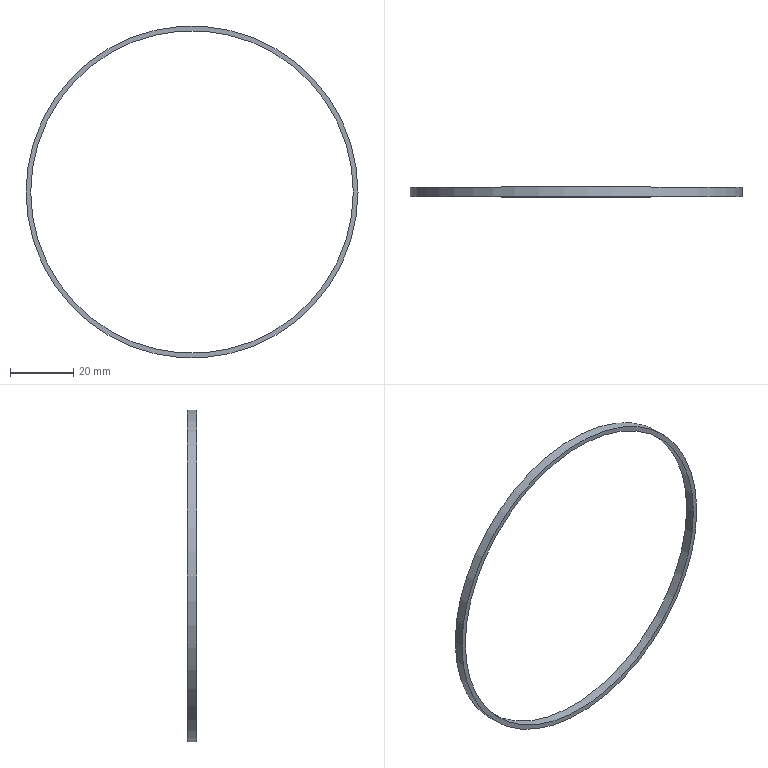Part | STEP file | 1-56.25 | 1 solid | 4 faces | box 105 x 3 x 105 mm | volume 1463 mm3 | plane 2 | cylinder 2 | commonest cylinder face diameters 102 x1 105 x1
STEP:
#1=CARTESIAN_POINT('',(0.,0.,0.));
#2=DIRECTION('',(0.,0.,1.));
#3=DIRECTION('',(1.,0.,0.));
#4=AXIS2_PLACEMENT_3D('',#1,#2,#3);
#5=CARTESIAN_POINT('',(52.5,0.,0.));
#6=VERTEX_POINT('',#5);
#7=CARTESIAN_POINT('',(0.,0.,0.));
#8=DIRECTION('',(0.,-1.,0.));
#9=DIRECTION('',(1.,0.,0.));
#10=AXIS2_PLACEMENT_3D('',#7,#8,#9);
#11=CIRCLE('',#10,52.5);
#12=CARTESIAN_POINT('',(-14.067,0.,0.));
#13=DIRECTION('',(0.,-1.,0.));
#14=DIRECTION('',(1.,0.,0.));
#15=AXIS2_PLACEMENT_3D('',#12,#13,#14);
#16=PLANE('',#15);
#17=CARTESIAN_POINT('',(14.067,0.));
#18=DIRECTION('',(1.,0.));
#19=AXIS2_PLACEMENT_2D('',#17,#18);
#20=CIRCLE('',#19,52.5);
#21=(GEOMETRIC_REPRESENTATION_CONTEXT(2)PARAMETRIC_REPRESENTATION_CONTEXT()REPRESENTATION_CONTEXT('',''));
#22=DEFINITIONAL_REPRESENTATION('',(#20),#21);
#23=PCURVE('',#16,#22);
#24=CARTESIAN_POINT('',(0.,0.,0.));
#25=DIRECTION('',(0.,-1.,0.));
#26=DIRECTION('',(1.,0.,0.));
#27=AXIS2_PLACEMENT_3D('',#24,#25,#26);
#28=CYLINDRICAL_SURFACE('',#27,52.5);
#29=CARTESIAN_POINT('',(0.,0.));
#30=DIRECTION('',(1.,0.));
#31=VECTOR('',#30,1.);
#32=LINE('',#29,#31);
#33=(GEOMETRIC_REPRESENTATION_CONTEXT(2)PARAMETRIC_REPRESENTATION_CONTEXT()REPRESENTATION_CONTEXT('',''));
#34=DEFINITIONAL_REPRESENTATION('',(#32),#33);
#35=PCURVE('',#28,#34);
#36=SURFACE_CURVE('',#11,(#23,#35),.PCURVE_S1.);
#37=EDGE_CURVE('',#6,#6,#36,.T.);
#38=ORIENTED_EDGE('',*,*,#37,.T.);
#39=EDGE_LOOP('',(#38));
#40=FACE_BOUND('',#39,.F.);
#41=CARTESIAN_POINT('',(51.,0.,0.));
#42=VERTEX_POINT('',#41);
#43=CARTESIAN_POINT('',(0.,0.,0.));
#44=DIRECTION('',(0.,1.,0.));
#45=DIRECTION('',(1.,0.,0.));
#46=AXIS2_PLACEMENT_3D('',#43,#44,#45);
#47=CIRCLE('',#46,51.);
#48=CARTESIAN_POINT('',(65.067,0.));
#49=CARTESIAN_POINT('',(65.067,-88.335));
#50=CARTESIAN_POINT('',(-11.433,-44.167));
#51=CARTESIAN_POINT('',(-87.933,0.));
#52=CARTESIAN_POINT('',(-11.433,44.167));
#53=CARTESIAN_POINT('',(65.067,88.335));
#54=CARTESIAN_POINT('',(65.067,0.));
#55=(BOUNDED_CURVE()B_SPLINE_CURVE(2,(#48,#49,#50,#51,#52,#53,#54),.UNSPECIFIED.,.T.,.F.)B_SPLINE_CURVE_WITH_KNOTS((1,2,2,2,2,1),(-2.094,0.,2.094,4.189,6.283,8.378),.UNSPECIFIED.)CURVE()GEOMETRIC_REPRESENTATION_ITEM()RATIONAL_B_SPLINE_CURVE((1.,0.5,1.,0.5,1.,0.5,1.))REPRESENTATION_ITEM(''));
#56=(GEOMETRIC_REPRESENTATION_CONTEXT(2)PARAMETRIC_REPRESENTATION_CONTEXT()REPRESENTATION_CONTEXT('',''));
#57=DEFINITIONAL_REPRESENTATION('',(#55),#56);
#58=PCURVE('',#16,#57);
#59=CARTESIAN_POINT('',(0.,0.,0.));
#60=DIRECTION('',(0.,-1.,0.));
#61=DIRECTION('',(1.,0.,0.));
#62=AXIS2_PLACEMENT_3D('',#59,#60,#61);
#63=CYLINDRICAL_SURFACE('',#62,51.);
#64=CARTESIAN_POINT('',(6.283,0.));
#65=DIRECTION('',(-1.,0.));
#66=VECTOR('',#65,1.);
#67=LINE('',#64,#66);
#68=(GEOMETRIC_REPRESENTATION_CONTEXT(2)PARAMETRIC_REPRESENTATION_CONTEXT()REPRESENTATION_CONTEXT('',''));
#69=DEFINITIONAL_REPRESENTATION('',(#67),#68);
#70=PCURVE('',#63,#69);
#71=SURFACE_CURVE('',#47,(#58,#70),.PCURVE_S1.);
#72=EDGE_CURVE('',#42,#42,#71,.T.);
#73=ORIENTED_EDGE('',*,*,#72,.T.);
#74=EDGE_LOOP('',(#73));
#75=FACE_BOUND('',#74,.F.);
#76=ADVANCED_FACE('',(#40,#75),#16,.F.);
#77=CARTESIAN_POINT('',(52.5,-3.,0.));
#78=VERTEX_POINT('',#77);
#79=CARTESIAN_POINT('',(0.,-3.,0.));
#80=DIRECTION('',(0.,-1.,0.));
#81=DIRECTION('',(1.,0.,0.));
#82=AXIS2_PLACEMENT_3D('',#79,#80,#81);
#83=CIRCLE('',#82,52.5);
#84=CARTESIAN_POINT('',(-14.067,-3.,0.));
#85=DIRECTION('',(0.,-1.,0.));
#86=DIRECTION('',(1.,0.,0.));
#87=AXIS2_PLACEMENT_3D('',#84,#85,#86);
#88=PLANE('',#87);
#89=CARTESIAN_POINT('',(14.067,0.));
#90=DIRECTION('',(1.,0.));
#91=AXIS2_PLACEMENT_2D('',#89,#90);
#92=CIRCLE('',#91,52.5);
#93=(GEOMETRIC_REPRESENTATION_CONTEXT(2)PARAMETRIC_REPRESENTATION_CONTEXT()REPRESENTATION_CONTEXT('',''));
#94=DEFINITIONAL_REPRESENTATION('',(#92),#93);
#95=PCURVE('',#88,#94);
#96=CARTESIAN_POINT('',(0.,3.));
#97=DIRECTION('',(1.,0.));
#98=VECTOR('',#97,1.);
#99=LINE('',#96,#98);
#100=(GEOMETRIC_REPRESENTATION_CONTEXT(2)PARAMETRIC_REPRESENTATION_CONTEXT()REPRESENTATION_CONTEXT('',''));
#101=DEFINITIONAL_REPRESENTATION('',(#99),#100);
#102=PCURVE('',#28,#101);
#103=SURFACE_CURVE('',#83,(#95,#102),.PCURVE_S1.);
#104=EDGE_CURVE('',#78,#78,#103,.T.);
#105=ORIENTED_EDGE('',*,*,#104,.T.);
#106=EDGE_LOOP('',(#105));
#107=FACE_BOUND('',#106,.T.);
#108=CARTESIAN_POINT('',(51.,-3.,0.));
#109=VERTEX_POINT('',#108);
#110=CARTESIAN_POINT('',(0.,-3.,0.));
#111=DIRECTION('',(0.,1.,0.));
#112=DIRECTION('',(1.,0.,0.));
#113=AXIS2_PLACEMENT_3D('',#110,#111,#112);
#114=CIRCLE('',#113,51.);
#115=CARTESIAN_POINT('',(65.067,0.));
#116=CARTESIAN_POINT('',(65.067,-88.335));
#117=CARTESIAN_POINT('',(-11.433,-44.167));
#118=CARTESIAN_POINT('',(-87.933,0.));
#119=CARTESIAN_POINT('',(-11.433,44.167));
#120=CARTESIAN_POINT('',(65.067,88.335));
#121=CARTESIAN_POINT('',(65.067,0.));
#122=(BOUNDED_CURVE()B_SPLINE_CURVE(2,(#115,#116,#117,#118,#119,#120,#121),.UNSPECIFIED.,.T.,.F.)B_SPLINE_CURVE_WITH_KNOTS((1,2,2,2,2,1),(-2.094,0.,2.094,4.189,6.283,8.378),.UNSPECIFIED.)CURVE()GEOMETRIC_REPRESENTATION_ITEM()RATIONAL_B_SPLINE_CURVE((1.,0.5,1.,0.5,1.,0.5,1.))REPRESENTATION_ITEM(''));
#123=(GEOMETRIC_REPRESENTATION_CONTEXT(2)PARAMETRIC_REPRESENTATION_CONTEXT()REPRESENTATION_CONTEXT('',''));
#124=DEFINITIONAL_REPRESENTATION('',(#122),#123);
#125=PCURVE('',#88,#124);
#126=CARTESIAN_POINT('',(6.283,3.));
#127=DIRECTION('',(-1.,0.));
#128=VECTOR('',#127,1.);
#129=LINE('',#126,#128);
#130=(GEOMETRIC_REPRESENTATION_CONTEXT(2)PARAMETRIC_REPRESENTATION_CONTEXT()REPRESENTATION_CONTEXT('',''));
#131=DEFINITIONAL_REPRESENTATION('',(#129),#130);
#132=PCURVE('',#63,#131);
#133=SURFACE_CURVE('',#114,(#125,#132),.PCURVE_S1.);
#134=EDGE_CURVE('',#109,#109,#133,.T.);
#135=ORIENTED_EDGE('',*,*,#134,.T.);
#136=EDGE_LOOP('',(#135));
#137=FACE_BOUND('',#136,.T.);
#138=ADVANCED_FACE('',(#107,#137),#88,.T.);
#139=ORIENTED_EDGE('',*,*,#37,.T.);
#140=CARTESIAN_POINT('',(52.5,0.,0.));
#141=DIRECTION('',(0.,-1.,0.));
#142=VECTOR('',#141,1.);
#143=LINE('',#140,#142);
#144=CARTESIAN_POINT('',(6.283,0.));
#145=DIRECTION('',(0.,1.));
#146=VECTOR('',#145,1.);
#147=LINE('',#144,#146);
#148=(GEOMETRIC_REPRESENTATION_CONTEXT(2)PARAMETRIC_REPRESENTATION_CONTEXT()REPRESENTATION_CONTEXT('',''));
#149=DEFINITIONAL_REPRESENTATION('',(#147),#148);
#150=PCURVE('',#28,#149);
#151=CARTESIAN_POINT('',(0.,0.));
#152=DIRECTION('',(0.,1.));
#153=VECTOR('',#152,1.);
#154=LINE('',#151,#153);
#155=(GEOMETRIC_REPRESENTATION_CONTEXT(2)PARAMETRIC_REPRESENTATION_CONTEXT()REPRESENTATION_CONTEXT('',''));
#156=DEFINITIONAL_REPRESENTATION('',(#154),#155);
#157=PCURVE('',#28,#156);
#158=SEAM_CURVE('',#143,(#150,#157),.PCURVE_S1.);
#159=EDGE_CURVE('',#6,#78,#158,.T.);
#160=ORIENTED_EDGE('',*,*,#159,.T.);
#161=ORIENTED_EDGE('',*,*,#104,.F.);
#162=ORIENTED_EDGE('',*,*,#159,.F.);
#163=EDGE_LOOP('',(#139,#160,#161,#162));
#164=FACE_BOUND('',#163,.T.);
#165=ADVANCED_FACE('',(#164),#28,.T.);
#166=CARTESIAN_POINT('',(51.,0.,0.));
#167=DIRECTION('',(0.,-1.,0.));
#168=VECTOR('',#167,1.);
#169=LINE('',#166,#168);
#170=CARTESIAN_POINT('',(6.283,0.));
#171=DIRECTION('',(0.,1.));
#172=VECTOR('',#171,1.);
#173=LINE('',#170,#172);
#174=(GEOMETRIC_REPRESENTATION_CONTEXT(2)PARAMETRIC_REPRESENTATION_CONTEXT()REPRESENTATION_CONTEXT('',''));
#175=DEFINITIONAL_REPRESENTATION('',(#173),#174);
#176=PCURVE('',#63,#175);
#177=CARTESIAN_POINT('',(0.,0.));
#178=DIRECTION('',(0.,1.));
#179=VECTOR('',#178,1.);
#180=LINE('',#177,#179);
#181=(GEOMETRIC_REPRESENTATION_CONTEXT(2)PARAMETRIC_REPRESENTATION_CONTEXT()REPRESENTATION_CONTEXT('',''));
#182=DEFINITIONAL_REPRESENTATION('',(#180),#181);
#183=PCURVE('',#63,#182);
#184=SEAM_CURVE('',#169,(#176,#183),.PCURVE_S1.);
#185=EDGE_CURVE('',#42,#109,#184,.T.);
#186=ORIENTED_EDGE('',*,*,#185,.T.);
#187=ORIENTED_EDGE('',*,*,#134,.T.);
#188=ORIENTED_EDGE('',*,*,#185,.F.);
#189=ORIENTED_EDGE('',*,*,#72,.F.);
#190=EDGE_LOOP('',(#186,#187,#188,#189));
#191=FACE_BOUND('',#190,.F.);
#192=ADVANCED_FACE('',(#191),#63,.F.);
#193=CLOSED_SHELL('',(#76,#138,#165,#192));
#194=MANIFOLD_SOLID_BREP('',#193);
#195=(LENGTH_UNIT()NAMED_UNIT(*)SI_UNIT(.MILLI.,.METRE.));
#196=UNCERTAINTY_MEASURE_WITH_UNIT(LENGTH_MEASURE(0.0000001),#195,'','');
#197=(NAMED_UNIT(*)PLANE_ANGLE_UNIT()SI_UNIT($,.RADIAN.));
#198=(NAMED_UNIT(*)SI_UNIT($,.STERADIAN.)SOLID_ANGLE_UNIT());
#199=(GEOMETRIC_REPRESENTATION_CONTEXT(3)GLOBAL_UNCERTAINTY_ASSIGNED_CONTEXT((#196))GLOBAL_UNIT_ASSIGNED_CONTEXT((#195,#197,#198))REPRESENTATION_CONTEXT('',''));
#200=ADVANCED_BREP_SHAPE_REPRESENTATION('',(#4,#194),#199);